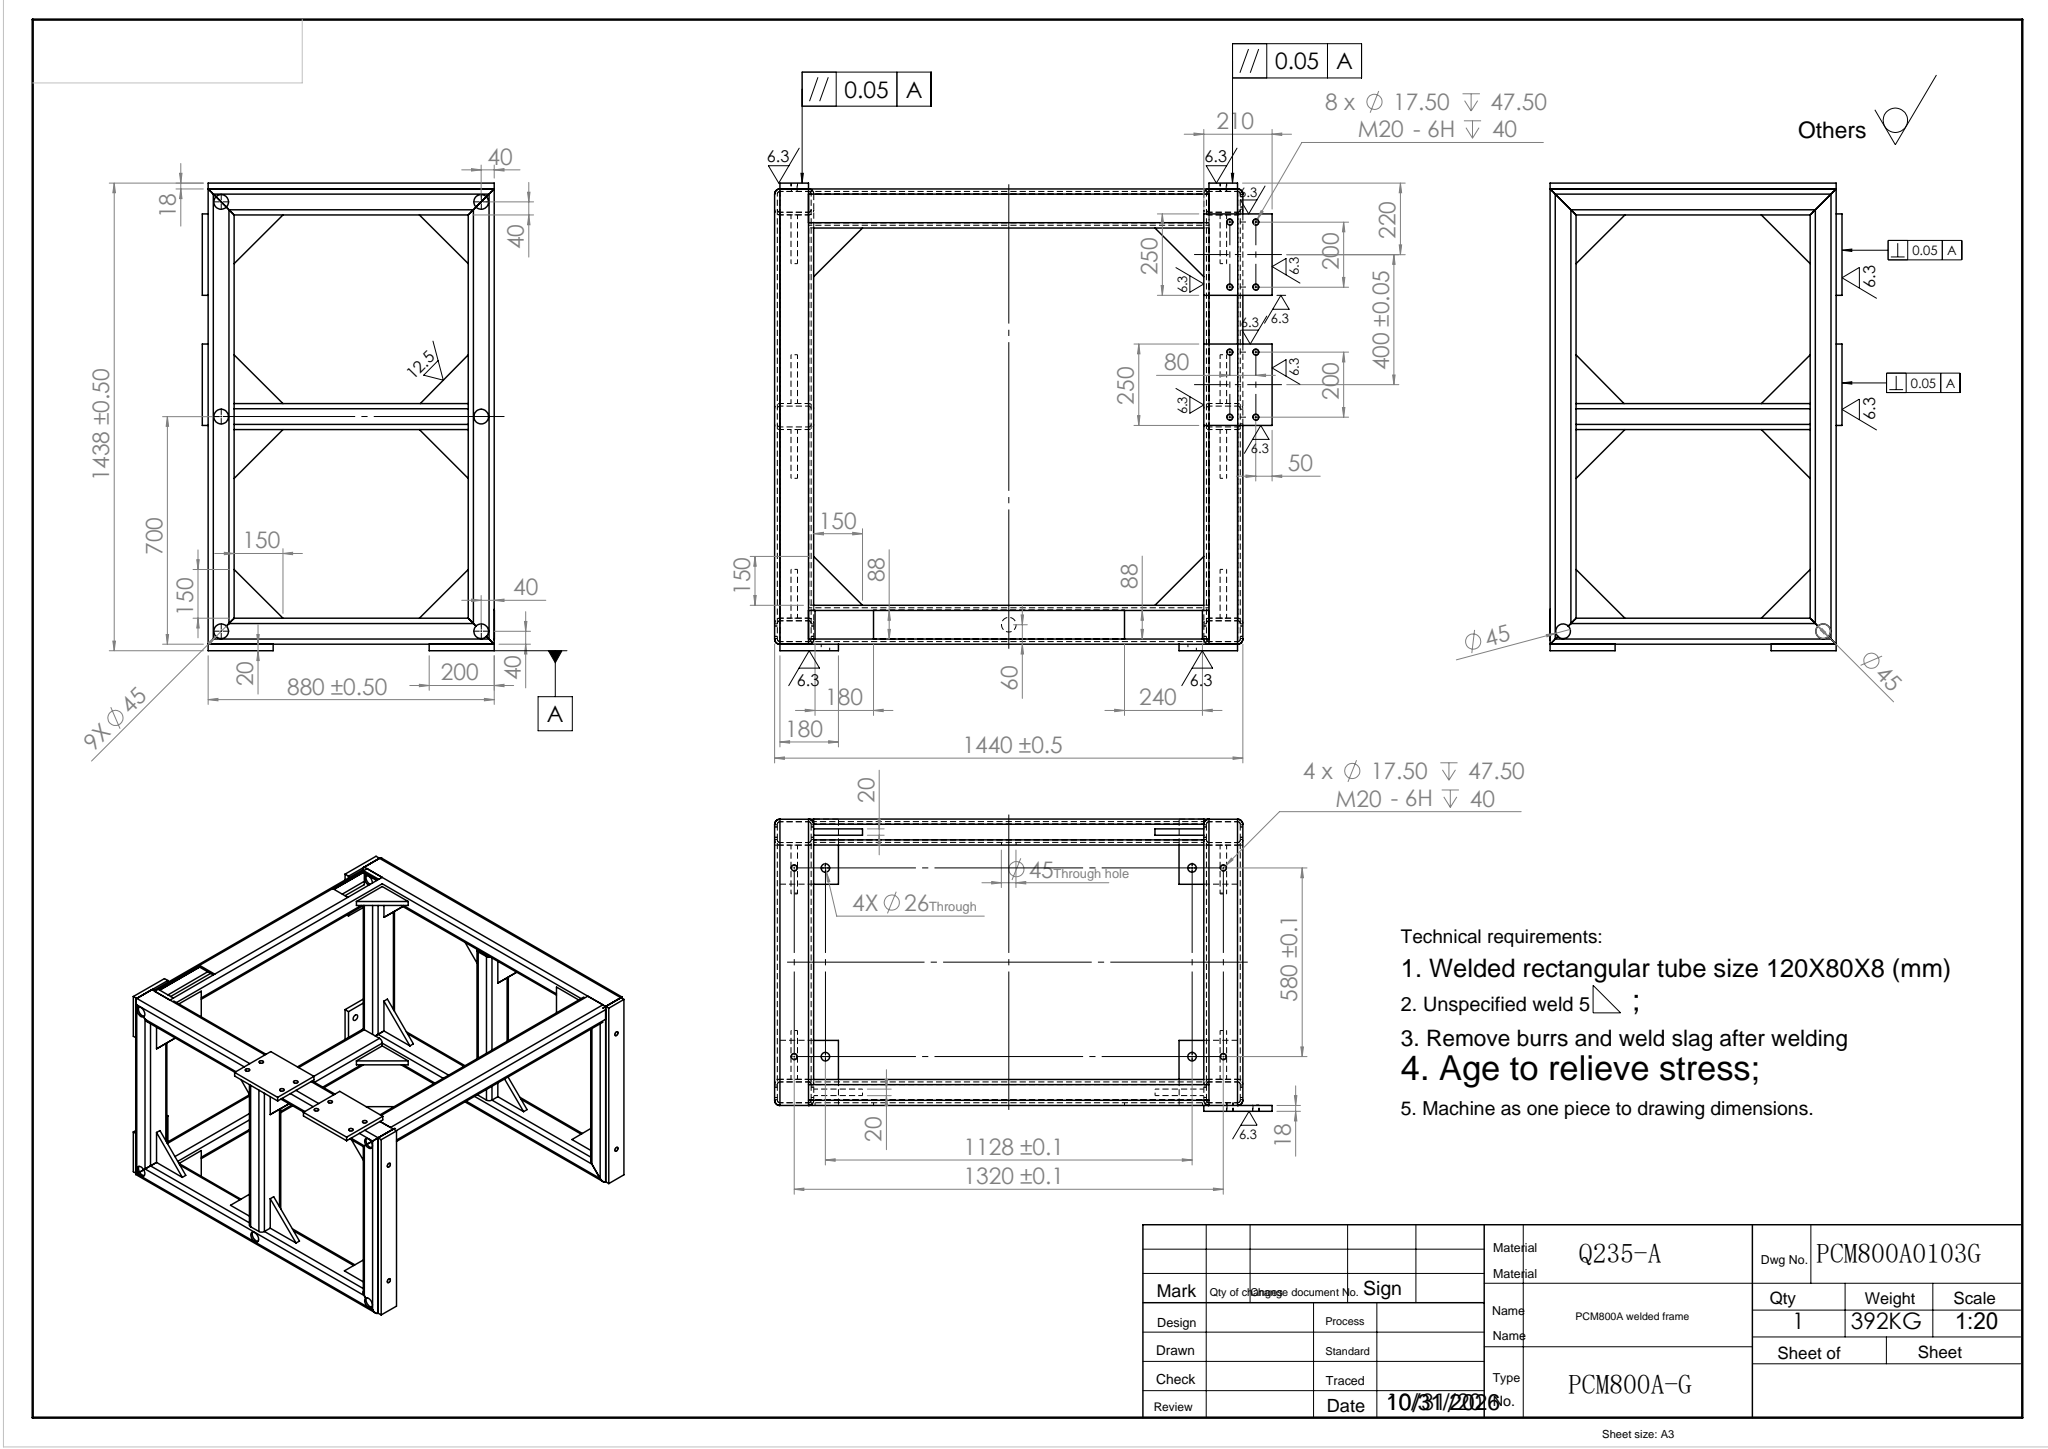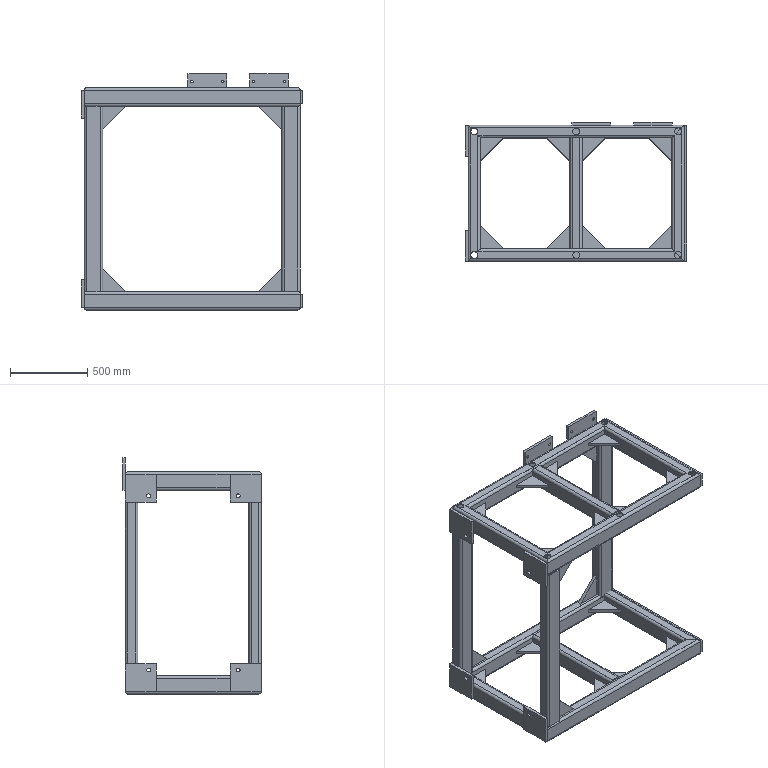Part | SolidWorks | features ICE 6, Boss 5, MirrorPattern 4, WeldMemberFeat 3, HoleWzd 2, LPattern 2, MirrorSolid 2, 3DProfileFeature 1, Cut 1, WeldmentFeature 1 | 35 solids | 484 faces | box 1438 x 898.415 x 1530 mm | volume 49681845 mm3 | plane 296 | cylinder 188 | commonest cylinder face diameters 16 x52 32 x52 17.5 x40 45 x36 26 x8